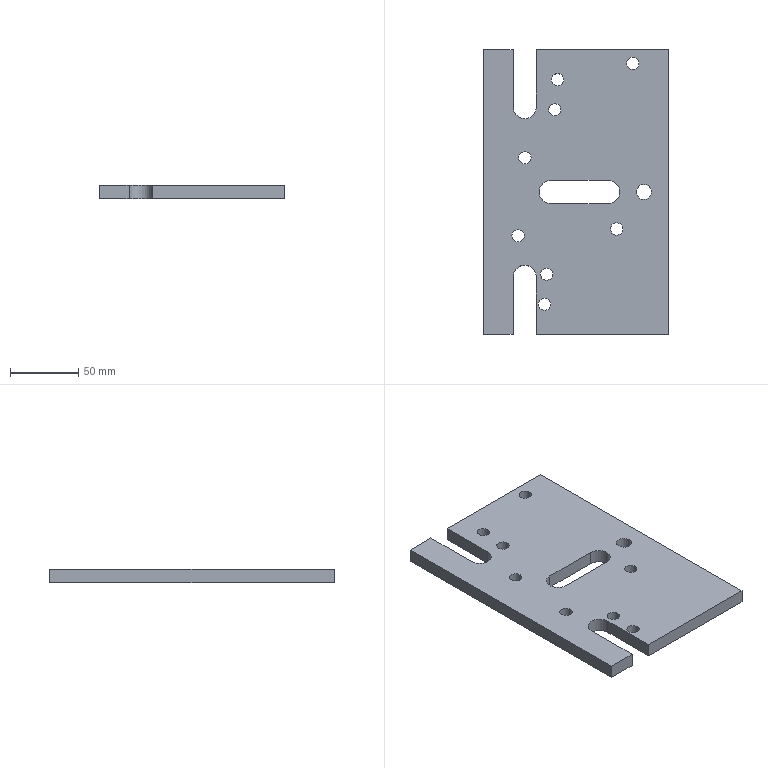Part | NX | features solid 2 | 1 solid | 27 faces | box 135 x 208 x 10 mm | volume 248801 mm3 | plane 14 | cylinder 13 | commonest cylinder face diameters 9 x8 17 x4 11 x1
STEP:
#1=CARTESIAN_POINT('',(374.5,-104.,-46.5));
#2=VERTEX_POINT('',#1);
#3=CARTESIAN_POINT('',(353.,-104.,-46.5));
#4=VERTEX_POINT('',#3);
#5=CARTESIAN_POINT('',(419.237,-104.,-46.5));
#6=DIRECTION('',(-1.,0.,0.));
#7=VECTOR('',#6,1000.);
#8=LINE('',#5,#7);
#9=EDGE_CURVE('',#2,#4,#8,.T.);
#10=ORIENTED_EDGE('',*,*,#9,.F.);
#11=CARTESIAN_POINT('',(374.5,-104.,-36.5));
#12=VERTEX_POINT('',#11);
#13=CARTESIAN_POINT('',(374.5,-104.,-41.5));
#14=DIRECTION('',(0.,0.,-1.));
#15=VECTOR('',#14,1000.);
#16=LINE('',#13,#15);
#17=EDGE_CURVE('',#12,#2,#16,.T.);
#18=ORIENTED_EDGE('',*,*,#17,.F.);
#19=CARTESIAN_POINT('',(353.,-104.,-36.5));
#20=VERTEX_POINT('',#19);
#21=CARTESIAN_POINT('',(419.237,-104.,-36.5));
#22=DIRECTION('',(-1.,0.,0.));
#23=VECTOR('',#22,1000.);
#24=LINE('',#21,#23);
#25=EDGE_CURVE('',#12,#20,#24,.T.);
#26=ORIENTED_EDGE('',*,*,#25,.T.);
#27=CARTESIAN_POINT('',(353.,-104.,-46.5));
#28=DIRECTION('',(0.,0.,1.));
#29=VECTOR('',#28,1000.);
#30=LINE('',#27,#29);
#31=EDGE_CURVE('',#4,#20,#30,.T.);
#32=ORIENTED_EDGE('',*,*,#31,.F.);
#33=EDGE_LOOP('',(#10,#18,#26,#32));
#34=FACE_BOUND('',#33,.T.);
#35=CARTESIAN_POINT('',(419.237,-104.,-46.5));
#36=DIRECTION('',(0.,1.,0.));
#37=DIRECTION('',(0.,0.,1.));
#38=AXIS2_PLACEMENT_3D('',#35,#36,#37);
#39=PLANE('',#38);
#40=ADVANCED_FACE('',(#34),#39,.F.);
#41=CARTESIAN_POINT('',(391.5,104.,-46.5));
#42=VERTEX_POINT('',#41);
#43=CARTESIAN_POINT('',(488.,104.,-46.5));
#44=VERTEX_POINT('',#43);
#45=CARTESIAN_POINT('',(419.237,104.,-46.5));
#46=DIRECTION('',(1.,0.,0.));
#47=VECTOR('',#46,1000.);
#48=LINE('',#45,#47);
#49=EDGE_CURVE('',#42,#44,#48,.T.);
#50=ORIENTED_EDGE('',*,*,#49,.F.);
#51=CARTESIAN_POINT('',(391.5,104.,-36.5));
#52=VERTEX_POINT('',#51);
#53=CARTESIAN_POINT('',(391.5,104.,-46.5));
#54=DIRECTION('',(0.,0.,1.));
#55=VECTOR('',#54,1000.);
#56=LINE('',#53,#55);
#57=EDGE_CURVE('',#42,#52,#56,.T.);
#58=ORIENTED_EDGE('',*,*,#57,.T.);
#59=CARTESIAN_POINT('',(488.,104.,-36.5));
#60=VERTEX_POINT('',#59);
#61=CARTESIAN_POINT('',(419.237,104.,-36.5));
#62=DIRECTION('',(1.,0.,0.));
#63=VECTOR('',#62,1000.);
#64=LINE('',#61,#63);
#65=EDGE_CURVE('',#52,#60,#64,.T.);
#66=ORIENTED_EDGE('',*,*,#65,.T.);
#67=CARTESIAN_POINT('',(488.,104.,-46.5));
#68=DIRECTION('',(0.,0.,1.));
#69=VECTOR('',#68,1000.);
#70=LINE('',#67,#69);
#71=EDGE_CURVE('',#44,#60,#70,.T.);
#72=ORIENTED_EDGE('',*,*,#71,.F.);
#73=EDGE_LOOP('',(#50,#58,#66,#72));
#74=FACE_BOUND('',#73,.T.);
#75=CARTESIAN_POINT('',(419.237,104.,-46.5));
#76=DIRECTION('',(0.,-1.,0.));
#77=DIRECTION('',(0.,0.,-1.));
#78=AXIS2_PLACEMENT_3D('',#75,#76,#77);
#79=PLANE('',#78);
#80=ADVANCED_FACE('',(#74),#79,.F.);
#81=CARTESIAN_POINT('',(353.,104.,-36.5));
#82=VERTEX_POINT('',#81);
#83=CARTESIAN_POINT('',(353.,105.,-36.5));
#84=DIRECTION('',(0.,1.,0.));
#85=VECTOR('',#84,1000.);
#86=LINE('',#83,#85);
#87=EDGE_CURVE('',#82,#20,#86,.F.);
#88=ORIENTED_EDGE('',*,*,#87,.F.);
#89=CARTESIAN_POINT('',(353.,104.,-46.5));
#90=VERTEX_POINT('',#89);
#91=CARTESIAN_POINT('',(353.,104.,-46.5));
#92=DIRECTION('',(0.,0.,1.));
#93=VECTOR('',#92,1000.);
#94=LINE('',#91,#93);
#95=EDGE_CURVE('',#90,#82,#94,.T.);
#96=ORIENTED_EDGE('',*,*,#95,.F.);
#97=CARTESIAN_POINT('',(353.,105.,-46.5));
#98=DIRECTION('',(0.,1.,0.));
#99=VECTOR('',#98,1000.);
#100=LINE('',#97,#99);
#101=EDGE_CURVE('',#90,#4,#100,.F.);
#102=ORIENTED_EDGE('',*,*,#101,.T.);
#103=ORIENTED_EDGE('',*,*,#31,.T.);
#104=EDGE_LOOP('',(#88,#96,#102,#103));
#105=FACE_BOUND('',#104,.T.);
#106=CARTESIAN_POINT('',(353.,105.,-46.5));
#107=DIRECTION('',(-1.,0.,0.));
#108=DIRECTION('',(0.,0.,1.));
#109=AXIS2_PLACEMENT_3D('',#106,#107,#108);
#110=PLANE('',#109);
#111=ADVANCED_FACE('',(#105),#110,.T.);
#112=CARTESIAN_POINT('',(374.5,104.,-36.5));
#113=VERTEX_POINT('',#112);
#114=CARTESIAN_POINT('',(419.237,104.,-36.5));
#115=DIRECTION('',(1.,0.,0.));
#116=VECTOR('',#115,1000.);
#117=LINE('',#114,#116);
#118=EDGE_CURVE('',#82,#113,#117,.T.);
#119=ORIENTED_EDGE('',*,*,#118,.T.);
#120=CARTESIAN_POINT('',(374.5,104.,-46.5));
#121=VERTEX_POINT('',#120);
#122=CARTESIAN_POINT('',(374.5,104.,-46.5));
#123=DIRECTION('',(0.,0.,-1.));
#124=VECTOR('',#123,1000.);
#125=LINE('',#122,#124);
#126=EDGE_CURVE('',#113,#121,#125,.T.);
#127=ORIENTED_EDGE('',*,*,#126,.T.);
#128=CARTESIAN_POINT('',(419.237,104.,-46.5));
#129=DIRECTION('',(1.,0.,0.));
#130=VECTOR('',#129,1000.);
#131=LINE('',#128,#130);
#132=EDGE_CURVE('',#90,#121,#131,.T.);
#133=ORIENTED_EDGE('',*,*,#132,.F.);
#134=ORIENTED_EDGE('',*,*,#95,.T.);
#135=EDGE_LOOP('',(#119,#127,#133,#134));
#136=FACE_BOUND('',#135,.T.);
#137=CARTESIAN_POINT('',(419.237,104.,-46.5));
#138=DIRECTION('',(0.,-1.,0.));
#139=DIRECTION('',(0.,0.,-1.));
#140=AXIS2_PLACEMENT_3D('',#137,#138,#139);
#141=PLANE('',#140);
#142=ADVANCED_FACE('',(#136),#141,.F.);
#143=CARTESIAN_POINT('',(488.,-104.,-36.5));
#144=VERTEX_POINT('',#143);
#145=CARTESIAN_POINT('',(488.,108.,-36.5));
#146=DIRECTION('',(0.,1.,0.));
#147=VECTOR('',#146,1000.);
#148=LINE('',#145,#147);
#149=EDGE_CURVE('',#144,#60,#148,.T.);
#150=ORIENTED_EDGE('',*,*,#149,.F.);
#151=CARTESIAN_POINT('',(488.,-104.,-46.5));
#152=VERTEX_POINT('',#151);
#153=CARTESIAN_POINT('',(488.,-104.,-46.5));
#154=DIRECTION('',(0.,0.,1.));
#155=VECTOR('',#154,1000.);
#156=LINE('',#153,#155);
#157=EDGE_CURVE('',#152,#144,#156,.T.);
#158=ORIENTED_EDGE('',*,*,#157,.F.);
#159=CARTESIAN_POINT('',(488.,108.,-46.5));
#160=DIRECTION('',(0.,1.,0.));
#161=VECTOR('',#160,1000.);
#162=LINE('',#159,#161);
#163=EDGE_CURVE('',#152,#44,#162,.T.);
#164=ORIENTED_EDGE('',*,*,#163,.T.);
#165=ORIENTED_EDGE('',*,*,#71,.T.);
#166=EDGE_LOOP('',(#150,#158,#164,#165));
#167=FACE_BOUND('',#166,.T.);
#168=CARTESIAN_POINT('',(488.,108.,-46.5));
#169=DIRECTION('',(1.,0.,0.));
#170=DIRECTION('',(0.,0.,-1.));
#171=AXIS2_PLACEMENT_3D('',#168,#169,#170);
#172=PLANE('',#171);
#173=ADVANCED_FACE('',(#167),#172,.T.);
#174=CARTESIAN_POINT('',(464.5,0.,-46.5));
#175=VERTEX_POINT('',#174);
#176=CARTESIAN_POINT('',(470.,0.,-46.5));
#177=DIRECTION('',(0.,0.,-1.));
#178=DIRECTION('',(-1.,0.,0.));
#179=AXIS2_PLACEMENT_3D('',#176,#177,#178);
#180=CIRCLE('',#179,5.5);
#181=EDGE_CURVE('',#175,#175,#180,.T.);
#182=ORIENTED_EDGE('',*,*,#181,.T.);
#183=EDGE_LOOP('',(#182));
#184=FACE_BOUND('',#183,.T.);
#185=CARTESIAN_POINT('',(464.5,0.,-36.5));
#186=VERTEX_POINT('',#185);
#187=CARTESIAN_POINT('',(470.,0.,-36.5));
#188=DIRECTION('',(0.,0.,-1.));
#189=DIRECTION('',(-1.,0.,0.));
#190=AXIS2_PLACEMENT_3D('',#187,#188,#189);
#191=CIRCLE('',#190,5.5);
#192=EDGE_CURVE('',#186,#186,#191,.T.);
#193=ORIENTED_EDGE('',*,*,#192,.F.);
#194=EDGE_LOOP('',(#193));
#195=FACE_BOUND('',#194,.T.);
#196=CARTESIAN_POINT('',(470.,0.,-46.5));
#197=DIRECTION('',(0.,0.,1.));
#198=DIRECTION('',(1.,0.,0.));
#199=AXIS2_PLACEMENT_3D('',#196,#197,#198);
#200=CYLINDRICAL_SURFACE('',#199,5.5);
#201=ADVANCED_FACE('',(#184,#195),#200,.F.);
#202=CARTESIAN_POINT('',(457.5,94.003,-46.5));
#203=VERTEX_POINT('',#202);
#204=CARTESIAN_POINT('',(462.,94.003,-46.5));
#205=DIRECTION('',(0.,0.,-1.));
#206=DIRECTION('',(-1.,0.,0.));
#207=AXIS2_PLACEMENT_3D('',#204,#205,#206);
#208=CIRCLE('',#207,4.5);
#209=EDGE_CURVE('',#203,#203,#208,.T.);
#210=ORIENTED_EDGE('',*,*,#209,.T.);
#211=EDGE_LOOP('',(#210));
#212=FACE_BOUND('',#211,.T.);
#213=CARTESIAN_POINT('',(457.5,94.003,-36.5));
#214=VERTEX_POINT('',#213);
#215=CARTESIAN_POINT('',(462.,94.003,-36.5));
#216=DIRECTION('',(0.,0.,-1.));
#217=DIRECTION('',(-1.,0.,0.));
#218=AXIS2_PLACEMENT_3D('',#215,#216,#217);
#219=CIRCLE('',#218,4.5);
#220=EDGE_CURVE('',#214,#214,#219,.T.);
#221=ORIENTED_EDGE('',*,*,#220,.F.);
#222=EDGE_LOOP('',(#221));
#223=FACE_BOUND('',#222,.T.);
#224=CARTESIAN_POINT('',(462.,94.003,-46.5));
#225=DIRECTION('',(0.,0.,1.));
#226=DIRECTION('',(1.,0.,0.));
#227=AXIS2_PLACEMENT_3D('',#224,#225,#226);
#228=CYLINDRICAL_SURFACE('',#227,4.5);
#229=ADVANCED_FACE('',(#212,#223),#228,.F.);
#230=CARTESIAN_POINT('',(402.5,82.003,-46.5));
#231=VERTEX_POINT('',#230);
#232=CARTESIAN_POINT('',(407.,82.003,-46.5));
#233=DIRECTION('',(0.,0.,-1.));
#234=DIRECTION('',(-1.,0.,0.));
#235=AXIS2_PLACEMENT_3D('',#232,#233,#234);
#236=CIRCLE('',#235,4.5);
#237=EDGE_CURVE('',#231,#231,#236,.T.);
#238=ORIENTED_EDGE('',*,*,#237,.T.);
#239=EDGE_LOOP('',(#238));
#240=FACE_BOUND('',#239,.T.);
#241=CARTESIAN_POINT('',(402.5,82.003,-36.5));
#242=VERTEX_POINT('',#241);
#243=CARTESIAN_POINT('',(407.,82.003,-36.5));
#244=DIRECTION('',(0.,0.,-1.));
#245=DIRECTION('',(-1.,0.,0.));
#246=AXIS2_PLACEMENT_3D('',#243,#244,#245);
#247=CIRCLE('',#246,4.5);
#248=EDGE_CURVE('',#242,#242,#247,.T.);
#249=ORIENTED_EDGE('',*,*,#248,.F.);
#250=EDGE_LOOP('',(#249));
#251=FACE_BOUND('',#250,.T.);
#252=CARTESIAN_POINT('',(407.,82.003,-46.5));
#253=DIRECTION('',(0.,0.,1.));
#254=DIRECTION('',(1.,0.,0.));
#255=AXIS2_PLACEMENT_3D('',#252,#253,#254);
#256=CYLINDRICAL_SURFACE('',#255,4.5);
#257=ADVANCED_FACE('',(#240,#251),#256,.F.);
#258=CARTESIAN_POINT('',(400.5,60.003,-46.5));
#259=VERTEX_POINT('',#258);
#260=CARTESIAN_POINT('',(405.,60.003,-46.5));
#261=DIRECTION('',(0.,0.,-1.));
#262=DIRECTION('',(-1.,0.,0.));
#263=AXIS2_PLACEMENT_3D('',#260,#261,#262);
#264=CIRCLE('',#263,4.5);
#265=EDGE_CURVE('',#259,#259,#264,.T.);
#266=ORIENTED_EDGE('',*,*,#265,.T.);
#267=EDGE_LOOP('',(#266));
#268=FACE_BOUND('',#267,.T.);
#269=CARTESIAN_POINT('',(400.5,60.003,-36.5));
#270=VERTEX_POINT('',#269);
#271=CARTESIAN_POINT('',(405.,60.003,-36.5));
#272=DIRECTION('',(0.,0.,-1.));
#273=DIRECTION('',(-1.,0.,0.));
#274=AXIS2_PLACEMENT_3D('',#271,#272,#273);
#275=CIRCLE('',#274,4.5);
#276=EDGE_CURVE('',#270,#270,#275,.T.);
#277=ORIENTED_EDGE('',*,*,#276,.F.);
#278=EDGE_LOOP('',(#277));
#279=FACE_BOUND('',#278,.T.);
#280=CARTESIAN_POINT('',(405.,60.003,-46.5));
#281=DIRECTION('',(0.,0.,1.));
#282=DIRECTION('',(1.,0.,0.));
#283=AXIS2_PLACEMENT_3D('',#280,#281,#282);
#284=CYLINDRICAL_SURFACE('',#283,4.5);
#285=ADVANCED_FACE('',(#268,#279),#284,.F.);
#286=CARTESIAN_POINT('',(378.66,25.,-46.5));
#287=VERTEX_POINT('',#286);
#288=CARTESIAN_POINT('',(383.16,25.,-46.5));
#289=DIRECTION('',(0.,0.,-1.));
#290=DIRECTION('',(-1.,0.,0.));
#291=AXIS2_PLACEMENT_3D('',#288,#289,#290);
#292=CIRCLE('',#291,4.5);
#293=EDGE_CURVE('',#287,#287,#292,.T.);
#294=ORIENTED_EDGE('',*,*,#293,.T.);
#295=EDGE_LOOP('',(#294));
#296=FACE_BOUND('',#295,.T.);
#297=CARTESIAN_POINT('',(378.66,25.,-36.5));
#298=VERTEX_POINT('',#297);
#299=CARTESIAN_POINT('',(383.16,25.,-36.5));
#300=DIRECTION('',(0.,0.,-1.));
#301=DIRECTION('',(-1.,0.,0.));
#302=AXIS2_PLACEMENT_3D('',#299,#300,#301);
#303=CIRCLE('',#302,4.5);
#304=EDGE_CURVE('',#298,#298,#303,.T.);
#305=ORIENTED_EDGE('',*,*,#304,.F.);
#306=EDGE_LOOP('',(#305));
#307=FACE_BOUND('',#306,.T.);
#308=CARTESIAN_POINT('',(383.16,25.,-46.5));
#309=DIRECTION('',(0.,0.,1.));
#310=DIRECTION('',(1.,0.,0.));
#311=AXIS2_PLACEMENT_3D('',#308,#309,#310);
#312=CYLINDRICAL_SURFACE('',#311,4.5);
#313=ADVANCED_FACE('',(#296,#307),#312,.F.);
#314=CARTESIAN_POINT('',(373.66,-32.,-46.5));
#315=VERTEX_POINT('',#314);
#316=CARTESIAN_POINT('',(378.16,-32.,-46.5));
#317=DIRECTION('',(0.,0.,-1.));
#318=DIRECTION('',(-1.,0.,0.));
#319=AXIS2_PLACEMENT_3D('',#316,#317,#318);
#320=CIRCLE('',#319,4.5);
#321=EDGE_CURVE('',#315,#315,#320,.T.);
#322=ORIENTED_EDGE('',*,*,#321,.T.);
#323=EDGE_LOOP('',(#322));
#324=FACE_BOUND('',#323,.T.);
#325=CARTESIAN_POINT('',(373.66,-32.,-36.5));
#326=VERTEX_POINT('',#325);
#327=CARTESIAN_POINT('',(378.16,-32.,-36.5));
#328=DIRECTION('',(0.,0.,-1.));
#329=DIRECTION('',(-1.,0.,0.));
#330=AXIS2_PLACEMENT_3D('',#327,#328,#329);
#331=CIRCLE('',#330,4.5);
#332=EDGE_CURVE('',#326,#326,#331,.T.);
#333=ORIENTED_EDGE('',*,*,#332,.F.);
#334=EDGE_LOOP('',(#333));
#335=FACE_BOUND('',#334,.T.);
#336=CARTESIAN_POINT('',(378.16,-32.,-46.5));
#337=DIRECTION('',(0.,0.,1.));
#338=DIRECTION('',(1.,0.,0.));
#339=AXIS2_PLACEMENT_3D('',#336,#337,#338);
#340=CYLINDRICAL_SURFACE('',#339,4.5);
#341=ADVANCED_FACE('',(#324,#335),#340,.F.);
#342=CARTESIAN_POINT('',(394.5,-60.,-46.5));
#343=VERTEX_POINT('',#342);
#344=CARTESIAN_POINT('',(399.,-60.,-46.5));
#345=DIRECTION('',(0.,0.,-1.));
#346=DIRECTION('',(-1.,0.,0.));
#347=AXIS2_PLACEMENT_3D('',#344,#345,#346);
#348=CIRCLE('',#347,4.5);
#349=EDGE_CURVE('',#343,#343,#348,.T.);
#350=ORIENTED_EDGE('',*,*,#349,.T.);
#351=EDGE_LOOP('',(#350));
#352=FACE_BOUND('',#351,.T.);
#353=CARTESIAN_POINT('',(394.5,-60.,-36.5));
#354=VERTEX_POINT('',#353);
#355=CARTESIAN_POINT('',(399.,-60.,-36.5));
#356=DIRECTION('',(0.,0.,-1.));
#357=DIRECTION('',(-1.,0.,0.));
#358=AXIS2_PLACEMENT_3D('',#355,#356,#357);
#359=CIRCLE('',#358,4.5);
#360=EDGE_CURVE('',#354,#354,#359,.T.);
#361=ORIENTED_EDGE('',*,*,#360,.F.);
#362=EDGE_LOOP('',(#361));
#363=FACE_BOUND('',#362,.T.);
#364=CARTESIAN_POINT('',(399.,-60.,-46.5));
#365=DIRECTION('',(0.,0.,1.));
#366=DIRECTION('',(1.,0.,0.));
#367=AXIS2_PLACEMENT_3D('',#364,#365,#366);
#368=CYLINDRICAL_SURFACE('',#367,4.5);
#369=ADVANCED_FACE('',(#352,#363),#368,.F.);
#370=CARTESIAN_POINT('',(393.,-82.,-46.5));
#371=VERTEX_POINT('',#370);
#372=CARTESIAN_POINT('',(397.5,-82.,-46.5));
#373=DIRECTION('',(0.,0.,-1.));
#374=DIRECTION('',(-1.,0.,0.));
#375=AXIS2_PLACEMENT_3D('',#372,#373,#374);
#376=CIRCLE('',#375,4.5);
#377=EDGE_CURVE('',#371,#371,#376,.T.);
#378=ORIENTED_EDGE('',*,*,#377,.T.);
#379=EDGE_LOOP('',(#378));
#380=FACE_BOUND('',#379,.T.);
#381=CARTESIAN_POINT('',(393.,-82.,-36.5));
#382=VERTEX_POINT('',#381);
#383=CARTESIAN_POINT('',(397.5,-82.,-36.5));
#384=DIRECTION('',(0.,0.,-1.));
#385=DIRECTION('',(-1.,0.,0.));
#386=AXIS2_PLACEMENT_3D('',#383,#384,#385);
#387=CIRCLE('',#386,4.5);
#388=EDGE_CURVE('',#382,#382,#387,.T.);
#389=ORIENTED_EDGE('',*,*,#388,.F.);
#390=EDGE_LOOP('',(#389));
#391=FACE_BOUND('',#390,.T.);
#392=CARTESIAN_POINT('',(397.5,-82.,-46.5));
#393=DIRECTION('',(0.,0.,1.));
#394=DIRECTION('',(1.,0.,0.));
#395=AXIS2_PLACEMENT_3D('',#392,#393,#394);
#396=CYLINDRICAL_SURFACE('',#395,4.5);
#397=ADVANCED_FACE('',(#380,#391),#396,.F.);
#398=CARTESIAN_POINT('',(445.66,-27.,-46.5));
#399=VERTEX_POINT('',#398);
#400=CARTESIAN_POINT('',(450.16,-27.,-46.5));
#401=DIRECTION('',(0.,0.,-1.));
#402=DIRECTION('',(-1.,0.,0.));
#403=AXIS2_PLACEMENT_3D('',#400,#401,#402);
#404=CIRCLE('',#403,4.5);
#405=EDGE_CURVE('',#399,#399,#404,.T.);
#406=ORIENTED_EDGE('',*,*,#405,.T.);
#407=EDGE_LOOP('',(#406));
#408=FACE_BOUND('',#407,.T.);
#409=CARTESIAN_POINT('',(445.66,-27.,-36.5));
#410=VERTEX_POINT('',#409);
#411=CARTESIAN_POINT('',(450.16,-27.,-36.5));
#412=DIRECTION('',(0.,0.,-1.));
#413=DIRECTION('',(-1.,0.,0.));
#414=AXIS2_PLACEMENT_3D('',#411,#412,#413);
#415=CIRCLE('',#414,4.5);
#416=EDGE_CURVE('',#410,#410,#415,.T.);
#417=ORIENTED_EDGE('',*,*,#416,.F.);
#418=EDGE_LOOP('',(#417));
#419=FACE_BOUND('',#418,.T.);
#420=CARTESIAN_POINT('',(450.16,-27.,-46.5));
#421=DIRECTION('',(0.,0.,1.));
#422=DIRECTION('',(1.,0.,0.));
#423=AXIS2_PLACEMENT_3D('',#420,#421,#422);
#424=CYLINDRICAL_SURFACE('',#423,4.5);
#425=ADVANCED_FACE('',(#408,#419),#424,.F.);
#426=CARTESIAN_POINT('',(391.5,-104.,-36.5));
#427=VERTEX_POINT('',#426);
#428=CARTESIAN_POINT('',(419.237,-104.,-36.5));
#429=DIRECTION('',(-1.,0.,0.));
#430=VECTOR('',#429,1000.);
#431=LINE('',#428,#430);
#432=EDGE_CURVE('',#144,#427,#431,.T.);
#433=ORIENTED_EDGE('',*,*,#432,.T.);
#434=CARTESIAN_POINT('',(391.5,-104.,-46.5));
#435=VERTEX_POINT('',#434);
#436=CARTESIAN_POINT('',(391.5,-104.,-41.5));
#437=DIRECTION('',(0.,0.,1.));
#438=VECTOR('',#437,1000.);
#439=LINE('',#436,#438);
#440=EDGE_CURVE('',#435,#427,#439,.T.);
#441=ORIENTED_EDGE('',*,*,#440,.F.);
#442=CARTESIAN_POINT('',(419.237,-104.,-46.5));
#443=DIRECTION('',(-1.,0.,0.));
#444=VECTOR('',#443,1000.);
#445=LINE('',#442,#444);
#446=EDGE_CURVE('',#152,#435,#445,.T.);
#447=ORIENTED_EDGE('',*,*,#446,.F.);
#448=ORIENTED_EDGE('',*,*,#157,.T.);
#449=EDGE_LOOP('',(#433,#441,#447,#448));
#450=FACE_BOUND('',#449,.T.);
#451=CARTESIAN_POINT('',(419.237,-104.,-46.5));
#452=DIRECTION('',(0.,1.,0.));
#453=DIRECTION('',(0.,0.,1.));
#454=AXIS2_PLACEMENT_3D('',#451,#452,#453);
#455=PLANE('',#454);
#456=ADVANCED_FACE('',(#450),#455,.F.);
#457=CARTESIAN_POINT('',(374.5,-62.,-46.5));
#458=VERTEX_POINT('',#457);
#459=CARTESIAN_POINT('',(374.5,0.,-46.5));
#460=DIRECTION('',(0.,1.,0.));
#461=VECTOR('',#460,1000.);
#462=LINE('',#459,#461);
#463=EDGE_CURVE('',#2,#458,#462,.T.);
#464=ORIENTED_EDGE('',*,*,#463,.F.);
#465=ORIENTED_EDGE('',*,*,#9,.T.);
#466=ORIENTED_EDGE('',*,*,#101,.F.);
#467=ORIENTED_EDGE('',*,*,#132,.T.);
#468=CARTESIAN_POINT('',(374.5,62.,-46.5));
#469=VERTEX_POINT('',#468);
#470=CARTESIAN_POINT('',(374.5,0.,-46.5));
#471=DIRECTION('',(0.,1.,0.));
#472=VECTOR('',#471,1000.);
#473=LINE('',#470,#472);
#474=EDGE_CURVE('',#469,#121,#473,.T.);
#475=ORIENTED_EDGE('',*,*,#474,.F.);
#476=CARTESIAN_POINT('',(391.5,62.,-46.5));
#477=VERTEX_POINT('',#476);
#478=CARTESIAN_POINT('',(383.,62.,-46.5));
#479=DIRECTION('',(0.,0.,-1.));
#480=DIRECTION('',(-1.,0.,0.));
#481=AXIS2_PLACEMENT_3D('',#478,#479,#480);
#482=CIRCLE('',#481,8.5);
#483=EDGE_CURVE('',#477,#469,#482,.T.);
#484=ORIENTED_EDGE('',*,*,#483,.F.);
#485=CARTESIAN_POINT('',(391.5,0.,-46.5));
#486=DIRECTION('',(0.,-1.,0.));
#487=VECTOR('',#486,1000.);
#488=LINE('',#485,#487);
#489=EDGE_CURVE('',#42,#477,#488,.T.);
#490=ORIENTED_EDGE('',*,*,#489,.F.);
#491=ORIENTED_EDGE('',*,*,#49,.T.);
#492=ORIENTED_EDGE('',*,*,#163,.F.);
#493=ORIENTED_EDGE('',*,*,#446,.T.);
#494=CARTESIAN_POINT('',(391.5,-62.,-46.5));
#495=VERTEX_POINT('',#494);
#496=CARTESIAN_POINT('',(391.5,0.,-46.5));
#497=DIRECTION('',(0.,-1.,0.));
#498=VECTOR('',#497,1000.);
#499=LINE('',#496,#498);
#500=EDGE_CURVE('',#495,#435,#499,.T.);
#501=ORIENTED_EDGE('',*,*,#500,.F.);
#502=CARTESIAN_POINT('',(383.,-62.,-46.5));
#503=DIRECTION('',(0.,0.,-1.));
#504=DIRECTION('',(-1.,0.,0.));
#505=AXIS2_PLACEMENT_3D('',#502,#503,#504);
#506=CIRCLE('',#505,8.5);
#507=EDGE_CURVE('',#458,#495,#506,.T.);
#508=ORIENTED_EDGE('',*,*,#507,.F.);
#509=EDGE_LOOP('',(#464,#465,#466,#467,#475,#484,#490,#491,#492,#493,#501,#508));
#510=FACE_BOUND('',#509,.T.);
#511=CARTESIAN_POINT('',(402.,-8.5,-46.5));
#512=VERTEX_POINT('',#511);
#513=CARTESIAN_POINT('',(402.,8.5,-46.5));
#514=VERTEX_POINT('',#513);
#515=CARTESIAN_POINT('',(402.,0.,-46.5));
#516=DIRECTION('',(0.,0.,-1.));
#517=DIRECTION('',(-1.,0.,0.));
#518=AXIS2_PLACEMENT_3D('',#515,#516,#517);
#519=CIRCLE('',#518,8.5);
#520=EDGE_CURVE('',#512,#514,#519,.T.);
#521=ORIENTED_EDGE('',*,*,#520,.F.);
#522=CARTESIAN_POINT('',(444.,-8.5,-46.5));
#523=VERTEX_POINT('',#522);
#524=CARTESIAN_POINT('',(419.237,-8.5,-46.5));
#525=DIRECTION('',(-1.,0.,0.));
#526=VECTOR('',#525,1000.);
#527=LINE('',#524,#526);
#528=EDGE_CURVE('',#523,#512,#527,.T.);
#529=ORIENTED_EDGE('',*,*,#528,.F.);
#530=CARTESIAN_POINT('',(444.,8.5,-46.5));
#531=VERTEX_POINT('',#530);
#532=CARTESIAN_POINT('',(444.,0.,-46.5));
#533=DIRECTION('',(0.,0.,-1.));
#534=DIRECTION('',(-1.,0.,0.));
#535=AXIS2_PLACEMENT_3D('',#532,#533,#534);
#536=CIRCLE('',#535,8.5);
#537=EDGE_CURVE('',#531,#523,#536,.T.);
#538=ORIENTED_EDGE('',*,*,#537,.F.);
#539=CARTESIAN_POINT('',(419.237,8.5,-46.5));
#540=DIRECTION('',(1.,0.,0.));
#541=VECTOR('',#540,1000.);
#542=LINE('',#539,#541);
#543=EDGE_CURVE('',#514,#531,#542,.T.);
#544=ORIENTED_EDGE('',*,*,#543,.F.);
#545=EDGE_LOOP('',(#521,#529,#538,#544));
#546=FACE_BOUND('',#545,.T.);
#547=ORIENTED_EDGE('',*,*,#405,.F.);
#548=EDGE_LOOP('',(#547));
#549=FACE_BOUND('',#548,.T.);
#550=ORIENTED_EDGE('',*,*,#377,.F.);
#551=EDGE_LOOP('',(#550));
#552=FACE_BOUND('',#551,.T.);
#553=ORIENTED_EDGE('',*,*,#349,.F.);
#554=EDGE_LOOP('',(#553));
#555=FACE_BOUND('',#554,.T.);
#556=ORIENTED_EDGE('',*,*,#321,.F.);
#557=EDGE_LOOP('',(#556));
#558=FACE_BOUND('',#557,.T.);
#559=ORIENTED_EDGE('',*,*,#293,.F.);
#560=EDGE_LOOP('',(#559));
#561=FACE_BOUND('',#560,.T.);
#562=ORIENTED_EDGE('',*,*,#265,.F.);
#563=EDGE_LOOP('',(#562));
#564=FACE_BOUND('',#563,.T.);
#565=ORIENTED_EDGE('',*,*,#237,.F.);
#566=EDGE_LOOP('',(#565));
#567=FACE_BOUND('',#566,.T.);
#568=ORIENTED_EDGE('',*,*,#209,.F.);
#569=EDGE_LOOP('',(#568));
#570=FACE_BOUND('',#569,.T.);
#571=ORIENTED_EDGE('',*,*,#181,.F.);
#572=EDGE_LOOP('',(#571));
#573=FACE_BOUND('',#572,.T.);
#574=CARTESIAN_POINT('',(419.237,0.,-46.5));
#575=DIRECTION('',(0.,0.,-1.));
#576=DIRECTION('',(-1.,0.,0.));
#577=AXIS2_PLACEMENT_3D('',#574,#575,#576);
#578=PLANE('',#577);
#579=ADVANCED_FACE('',(#510,#546,#549,#552,#555,#558,#561,#564,#567,#570,#573),#578,.T.);
#580=ORIENTED_EDGE('',*,*,#25,.F.);
#581=CARTESIAN_POINT('',(374.5,-62.,-36.5));
#582=VERTEX_POINT('',#581);
#583=CARTESIAN_POINT('',(374.5,0.,-36.5));
#584=DIRECTION('',(0.,1.,0.));
#585=VECTOR('',#584,1000.);
#586=LINE('',#583,#585);
#587=EDGE_CURVE('',#12,#582,#586,.T.);
#588=ORIENTED_EDGE('',*,*,#587,.T.);
#589=CARTESIAN_POINT('',(391.5,-62.,-36.5));
#590=VERTEX_POINT('',#589);
#591=CARTESIAN_POINT('',(383.,-62.,-36.5));
#592=DIRECTION('',(0.,0.,-1.));
#593=DIRECTION('',(-1.,0.,0.));
#594=AXIS2_PLACEMENT_3D('',#591,#592,#593);
#595=CIRCLE('',#594,8.5);
#596=EDGE_CURVE('',#582,#590,#595,.T.);
#597=ORIENTED_EDGE('',*,*,#596,.T.);
#598=CARTESIAN_POINT('',(391.5,0.,-36.5));
#599=DIRECTION('',(0.,-1.,0.));
#600=VECTOR('',#599,1000.);
#601=LINE('',#598,#600);
#602=EDGE_CURVE('',#590,#427,#601,.T.);
#603=ORIENTED_EDGE('',*,*,#602,.T.);
#604=ORIENTED_EDGE('',*,*,#432,.F.);
#605=ORIENTED_EDGE('',*,*,#149,.T.);
#606=ORIENTED_EDGE('',*,*,#65,.F.);
#607=CARTESIAN_POINT('',(391.5,62.,-36.5));
#608=VERTEX_POINT('',#607);
#609=CARTESIAN_POINT('',(391.5,0.,-36.5));
#610=DIRECTION('',(0.,-1.,0.));
#611=VECTOR('',#610,1000.);
#612=LINE('',#609,#611);
#613=EDGE_CURVE('',#52,#608,#612,.T.);
#614=ORIENTED_EDGE('',*,*,#613,.T.);
#615=CARTESIAN_POINT('',(374.5,62.,-36.5));
#616=VERTEX_POINT('',#615);
#617=CARTESIAN_POINT('',(383.,62.,-36.5));
#618=DIRECTION('',(0.,0.,-1.));
#619=DIRECTION('',(-1.,0.,0.));
#620=AXIS2_PLACEMENT_3D('',#617,#618,#619);
#621=CIRCLE('',#620,8.5);
#622=EDGE_CURVE('',#608,#616,#621,.T.);
#623=ORIENTED_EDGE('',*,*,#622,.T.);
#624=CARTESIAN_POINT('',(374.5,0.,-36.5));
#625=DIRECTION('',(0.,1.,0.));
#626=VECTOR('',#625,1000.);
#627=LINE('',#624,#626);
#628=EDGE_CURVE('',#616,#113,#627,.T.);
#629=ORIENTED_EDGE('',*,*,#628,.T.);
#630=ORIENTED_EDGE('',*,*,#118,.F.);
#631=ORIENTED_EDGE('',*,*,#87,.T.);
#632=EDGE_LOOP('',(#580,#588,#597,#603,#604,#605,#606,#614,#623,#629,#630,#631));
#633=FACE_BOUND('',#632,.T.);
#634=CARTESIAN_POINT('',(444.,-8.5,-36.5));
#635=VERTEX_POINT('',#634);
#636=CARTESIAN_POINT('',(402.,-8.5,-36.5));
#637=VERTEX_POINT('',#636);
#638=CARTESIAN_POINT('',(419.237,-8.5,-36.5));
#639=DIRECTION('',(-1.,0.,0.));
#640=VECTOR('',#639,1000.);
#641=LINE('',#638,#640);
#642=EDGE_CURVE('',#635,#637,#641,.T.);
#643=ORIENTED_EDGE('',*,*,#642,.T.);
#644=CARTESIAN_POINT('',(402.,8.5,-36.5));
#645=VERTEX_POINT('',#644);
#646=CARTESIAN_POINT('',(402.,0.,-36.5));
#647=DIRECTION('',(0.,0.,-1.));
#648=DIRECTION('',(-1.,0.,0.));
#649=AXIS2_PLACEMENT_3D('',#646,#647,#648);
#650=CIRCLE('',#649,8.5);
#651=EDGE_CURVE('',#637,#645,#650,.T.);
#652=ORIENTED_EDGE('',*,*,#651,.T.);
#653=CARTESIAN_POINT('',(444.,8.5,-36.5));
#654=VERTEX_POINT('',#653);
#655=CARTESIAN_POINT('',(419.237,8.5,-36.5));
#656=DIRECTION('',(1.,0.,0.));
#657=VECTOR('',#656,1000.);
#658=LINE('',#655,#657);
#659=EDGE_CURVE('',#645,#654,#658,.T.);
#660=ORIENTED_EDGE('',*,*,#659,.T.);
#661=CARTESIAN_POINT('',(444.,0.,-36.5));
#662=DIRECTION('',(0.,0.,-1.));
#663=DIRECTION('',(-1.,0.,0.));
#664=AXIS2_PLACEMENT_3D('',#661,#662,#663);
#665=CIRCLE('',#664,8.5);
#666=EDGE_CURVE('',#654,#635,#665,.T.);
#667=ORIENTED_EDGE('',*,*,#666,.T.);
#668=EDGE_LOOP('',(#643,#652,#660,#667));
#669=FACE_BOUND('',#668,.T.);
#670=ORIENTED_EDGE('',*,*,#416,.T.);
#671=EDGE_LOOP('',(#670));
#672=FACE_BOUND('',#671,.T.);
#673=ORIENTED_EDGE('',*,*,#388,.T.);
#674=EDGE_LOOP('',(#673));
#675=FACE_BOUND('',#674,.T.);
#676=ORIENTED_EDGE('',*,*,#360,.T.);
#677=EDGE_LOOP('',(#676));
#678=FACE_BOUND('',#677,.T.);
#679=ORIENTED_EDGE('',*,*,#332,.T.);
#680=EDGE_LOOP('',(#679));
#681=FACE_BOUND('',#680,.T.);
#682=ORIENTED_EDGE('',*,*,#304,.T.);
#683=EDGE_LOOP('',(#682));
#684=FACE_BOUND('',#683,.T.);
#685=ORIENTED_EDGE('',*,*,#276,.T.);
#686=EDGE_LOOP('',(#685));
#687=FACE_BOUND('',#686,.T.);
#688=ORIENTED_EDGE('',*,*,#248,.T.);
#689=EDGE_LOOP('',(#688));
#690=FACE_BOUND('',#689,.T.);
#691=ORIENTED_EDGE('',*,*,#220,.T.);
#692=EDGE_LOOP('',(#691));
#693=FACE_BOUND('',#692,.T.);
#694=ORIENTED_EDGE('',*,*,#192,.T.);
#695=EDGE_LOOP('',(#694));
#696=FACE_BOUND('',#695,.T.);
#697=CARTESIAN_POINT('',(419.237,0.,-36.5));
#698=DIRECTION('',(0.,0.,-1.));
#699=DIRECTION('',(-1.,0.,0.));
#700=AXIS2_PLACEMENT_3D('',#697,#698,#699);
#701=PLANE('',#700);
#702=ADVANCED_FACE('',(#633,#669,#672,#675,#678,#681,#684,#687,#690,#693,#696),#701,.F.);
#703=ORIENTED_EDGE('',*,*,#474,.T.);
#704=ORIENTED_EDGE('',*,*,#126,.F.);
#705=ORIENTED_EDGE('',*,*,#628,.F.);
#706=CARTESIAN_POINT('',(374.5,62.,-41.5));
#707=DIRECTION('',(0.,0.,-1.));
#708=VECTOR('',#707,1000.);
#709=LINE('',#706,#708);
#710=EDGE_CURVE('',#616,#469,#709,.T.);
#711=ORIENTED_EDGE('',*,*,#710,.T.);
#712=EDGE_LOOP('',(#703,#704,#705,#711));
#713=FACE_BOUND('',#712,.T.);
#714=CARTESIAN_POINT('',(374.5,83.,-41.5));
#715=DIRECTION('',(-1.,0.,0.));
#716=DIRECTION('',(0.,0.,-1.));
#717=AXIS2_PLACEMENT_3D('',#714,#715,#716);
#718=PLANE('',#717);
#719=ADVANCED_FACE('',(#713),#718,.F.);
#720=ORIENTED_EDGE('',*,*,#489,.T.);
#721=CARTESIAN_POINT('',(391.5,62.,-41.5));
#722=DIRECTION('',(0.,0.,1.));
#723=VECTOR('',#722,1000.);
#724=LINE('',#721,#723);
#725=EDGE_CURVE('',#477,#608,#724,.T.);
#726=ORIENTED_EDGE('',*,*,#725,.T.);
#727=ORIENTED_EDGE('',*,*,#613,.F.);
#728=ORIENTED_EDGE('',*,*,#57,.F.);
#729=EDGE_LOOP('',(#720,#726,#727,#728));
#730=FACE_BOUND('',#729,.T.);
#731=CARTESIAN_POINT('',(391.5,83.,-41.5));
#732=DIRECTION('',(1.,0.,0.));
#733=DIRECTION('',(0.,0.,1.));
#734=AXIS2_PLACEMENT_3D('',#731,#732,#733);
#735=PLANE('',#734);
#736=ADVANCED_FACE('',(#730),#735,.F.);
#737=ORIENTED_EDGE('',*,*,#483,.T.);
#738=ORIENTED_EDGE('',*,*,#710,.F.);
#739=ORIENTED_EDGE('',*,*,#622,.F.);
#740=ORIENTED_EDGE('',*,*,#725,.F.);
#741=EDGE_LOOP('',(#737,#738,#739,#740));
#742=FACE_BOUND('',#741,.T.);
#743=CARTESIAN_POINT('',(383.,62.,-41.5));
#744=DIRECTION('',(0.,0.,-1.));
#745=DIRECTION('',(1.,0.,0.));
#746=AXIS2_PLACEMENT_3D('',#743,#744,#745);
#747=CYLINDRICAL_SURFACE('',#746,8.5);
#748=ADVANCED_FACE('',(#742),#747,.F.);
#749=ORIENTED_EDGE('',*,*,#543,.T.);
#750=CARTESIAN_POINT('',(444.,8.5,-41.5));
#751=DIRECTION('',(0.,0.,-1.));
#752=VECTOR('',#751,1000.);
#753=LINE('',#750,#752);
#754=EDGE_CURVE('',#531,#654,#753,.F.);
#755=ORIENTED_EDGE('',*,*,#754,.T.);
#756=ORIENTED_EDGE('',*,*,#659,.F.);
#757=CARTESIAN_POINT('',(402.,8.5,-41.5));
#758=DIRECTION('',(0.,0.,-1.));
#759=VECTOR('',#758,1000.);
#760=LINE('',#757,#759);
#761=EDGE_CURVE('',#645,#514,#760,.T.);
#762=ORIENTED_EDGE('',*,*,#761,.T.);
#763=EDGE_LOOP('',(#749,#755,#756,#762));
#764=FACE_BOUND('',#763,.T.);
#765=CARTESIAN_POINT('',(423.,8.5,-41.5));
#766=DIRECTION('',(0.,1.,0.));
#767=DIRECTION('',(0.,0.,-1.));
#768=AXIS2_PLACEMENT_3D('',#765,#766,#767);
#769=PLANE('',#768);
#770=ADVANCED_FACE('',(#764),#769,.F.);
#771=ORIENTED_EDGE('',*,*,#528,.T.);
#772=CARTESIAN_POINT('',(402.,-8.5,-41.5));
#773=DIRECTION('',(0.,0.,1.));
#774=VECTOR('',#773,1000.);
#775=LINE('',#772,#774);
#776=EDGE_CURVE('',#512,#637,#775,.T.);
#777=ORIENTED_EDGE('',*,*,#776,.T.);
#778=ORIENTED_EDGE('',*,*,#642,.F.);
#779=CARTESIAN_POINT('',(444.,-8.5,-41.5));
#780=DIRECTION('',(0.,0.,1.));
#781=VECTOR('',#780,1000.);
#782=LINE('',#779,#781);
#783=EDGE_CURVE('',#635,#523,#782,.F.);
#784=ORIENTED_EDGE('',*,*,#783,.T.);
#785=EDGE_LOOP('',(#771,#777,#778,#784));
#786=FACE_BOUND('',#785,.T.);
#787=CARTESIAN_POINT('',(423.,-8.5,-41.5));
#788=DIRECTION('',(0.,-1.,0.));
#789=DIRECTION('',(0.,0.,1.));
#790=AXIS2_PLACEMENT_3D('',#787,#788,#789);
#791=PLANE('',#790);
#792=ADVANCED_FACE('',(#786),#791,.F.);
#793=ORIENTED_EDGE('',*,*,#520,.T.);
#794=ORIENTED_EDGE('',*,*,#761,.F.);
#795=ORIENTED_EDGE('',*,*,#651,.F.);
#796=ORIENTED_EDGE('',*,*,#776,.F.);
#797=EDGE_LOOP('',(#793,#794,#795,#796));
#798=FACE_BOUND('',#797,.T.);
#799=CARTESIAN_POINT('',(402.,0.,-41.5));
#800=DIRECTION('',(0.,0.,-1.));
#801=DIRECTION('',(0.,-1.,0.));
#802=AXIS2_PLACEMENT_3D('',#799,#800,#801);
#803=CYLINDRICAL_SURFACE('',#802,8.5);
#804=ADVANCED_FACE('',(#798),#803,.F.);
#805=ORIENTED_EDGE('',*,*,#537,.T.);
#806=ORIENTED_EDGE('',*,*,#783,.F.);
#807=ORIENTED_EDGE('',*,*,#666,.F.);
#808=ORIENTED_EDGE('',*,*,#754,.F.);
#809=EDGE_LOOP('',(#805,#806,#807,#808));
#810=FACE_BOUND('',#809,.T.);
#811=CARTESIAN_POINT('',(444.,0.,-41.5));
#812=DIRECTION('',(0.,0.,1.));
#813=DIRECTION('',(0.,1.,0.));
#814=AXIS2_PLACEMENT_3D('',#811,#812,#813);
#815=CYLINDRICAL_SURFACE('',#814,8.5);
#816=ADVANCED_FACE('',(#810),#815,.F.);
#817=ORIENTED_EDGE('',*,*,#463,.T.);
#818=CARTESIAN_POINT('',(374.5,-62.,-41.5));
#819=DIRECTION('',(0.,0.,-1.));
#820=VECTOR('',#819,1000.);
#821=LINE('',#818,#820);
#822=EDGE_CURVE('',#582,#458,#821,.T.);
#823=ORIENTED_EDGE('',*,*,#822,.F.);
#824=ORIENTED_EDGE('',*,*,#587,.F.);
#825=ORIENTED_EDGE('',*,*,#17,.T.);
#826=EDGE_LOOP('',(#817,#823,#824,#825));
#827=FACE_BOUND('',#826,.T.);
#828=CARTESIAN_POINT('',(374.5,-83.,-41.5));
#829=DIRECTION('',(-1.,0.,0.));
#830=DIRECTION('',(0.,0.,-1.));
#831=AXIS2_PLACEMENT_3D('',#828,#829,#830);
#832=PLANE('',#831);
#833=ADVANCED_FACE('',(#827),#832,.F.);
#834=ORIENTED_EDGE('',*,*,#500,.T.);
#835=ORIENTED_EDGE('',*,*,#440,.T.);
#836=ORIENTED_EDGE('',*,*,#602,.F.);
#837=CARTESIAN_POINT('',(391.5,-62.,-41.5));
#838=DIRECTION('',(0.,0.,-1.));
#839=VECTOR('',#838,1000.);
#840=LINE('',#837,#839);
#841=EDGE_CURVE('',#495,#590,#840,.F.);
#842=ORIENTED_EDGE('',*,*,#841,.F.);
#843=EDGE_LOOP('',(#834,#835,#836,#842));
#844=FACE_BOUND('',#843,.T.);
#845=CARTESIAN_POINT('',(391.5,-83.,-41.5));
#846=DIRECTION('',(1.,0.,0.));
#847=DIRECTION('',(0.,0.,1.));
#848=AXIS2_PLACEMENT_3D('',#845,#846,#847);
#849=PLANE('',#848);
#850=ADVANCED_FACE('',(#844),#849,.F.);
#851=ORIENTED_EDGE('',*,*,#507,.T.);
#852=ORIENTED_EDGE('',*,*,#841,.T.);
#853=ORIENTED_EDGE('',*,*,#596,.F.);
#854=ORIENTED_EDGE('',*,*,#822,.T.);
#855=EDGE_LOOP('',(#851,#852,#853,#854));
#856=FACE_BOUND('',#855,.T.);
#857=CARTESIAN_POINT('',(383.,-62.,-41.5));
#858=DIRECTION('',(0.,0.,-1.));
#859=DIRECTION('',(1.,0.,0.));
#860=AXIS2_PLACEMENT_3D('',#857,#858,#859);
#861=CYLINDRICAL_SURFACE('',#860,8.5);
#862=ADVANCED_FACE('',(#856),#861,.F.);
#863=CLOSED_SHELL('',(#40,#80,#111,#142,#173,#201,#229,#257,#285,#313,#341,#369,#397,#425,#456,#579,#702,#719,#736,#748,#770,#792,#804,#816,#833,#850,#862));
#864=MANIFOLD_SOLID_BREP('',#863);
#865=(LENGTH_UNIT()NAMED_UNIT(*)SI_UNIT(.MILLI.,.METRE.));
#866=UNCERTAINTY_MEASURE_WITH_UNIT(LENGTH_MEASURE(0.00001),#865,'','');
#867=(NAMED_UNIT(*)PLANE_ANGLE_UNIT()SI_UNIT($,.RADIAN.));
#868=(NAMED_UNIT(*)SI_UNIT($,.STERADIAN.)SOLID_ANGLE_UNIT());
#869=(GEOMETRIC_REPRESENTATION_CONTEXT(3)GLOBAL_UNCERTAINTY_ASSIGNED_CONTEXT((#866))GLOBAL_UNIT_ASSIGNED_CONTEXT((#865,#867,#868))REPRESENTATION_CONTEXT('',''));
#870=ADVANCED_BREP_SHAPE_REPRESENTATION('',(#864),#869);